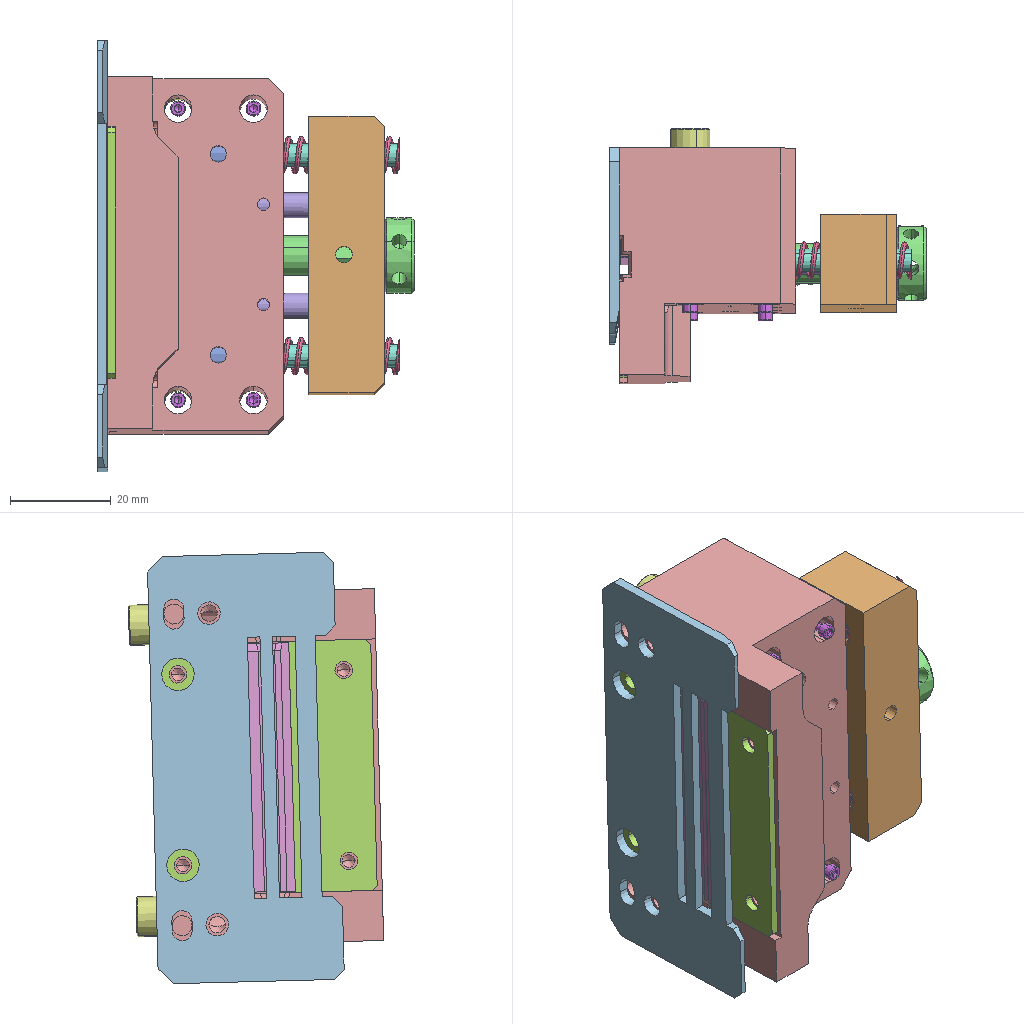Assembly | SolidWorks | 12 different items | 21 placed | box 63 x 51 x 86 mm
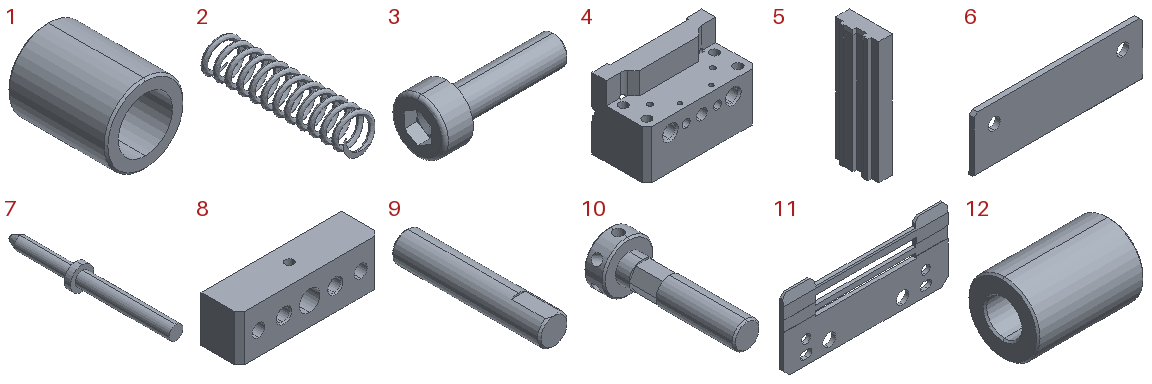Parts list (item | quantity | size | volume | features):
1 | x2 | 8 x 10 x 8 mm | 264.083 mm3 | features Chamfer 1, Extrusion 1
2 | x2 | 7.5 x 30 x 7.5 mm | 192.185 mm3 | features Helix 1, ICE 1, RefAxis 1, Sweep 1
3 | x4 | 7.6 x 3 x 3 mm | 21.652 mm3 | features Fillet 2, RevCut 2, Boss 1, Chamfer 1, Cut 1, Extrusion 1, LPattern 1
4 | x1 | 70 x 35 x 45 mm | 68698 mm3 | features ICE 23, Chamfer 5, HoleWzd 5, 3DProfileFeature 3, Cut 2, Extrusion 1, Fillet 1, LPattern 1, MirrorPattern 1
5 | x1 | 7 x 17.4 x 49.4 mm | 5230 mm3 | features ICE 3, Chamfer 2, RefAxis 2, Extrusion 1, MirrorPattern 1, RevCut 1
6 | x2 | 50 x 1.5 x 16.3 mm | 1186 mm3 | features Chamfer 2, Extrusion 1, ICE 1
7 | x2 | 7.5 x 53 x 7.5 mm | 808.158 mm3 | features ICE 3, Revolution 2, Extrusion 1, RefAxis 1, RevCut 1
8 | x1 | 55 x 15 x 18 mm | 12154 mm3 | features ICE 9, Chamfer 3, 3DProfileFeature 2, HoleWzd 2, Extrusion 1
9 | x2 | 5 x 25 x 5 mm | 486.718 mm3 | features Chamfer 1, Extrusion 1, ICE 1
10 | x1 | 15 x 41 x 15 mm | 2454 mm3 | features ICE 3, CirPattern 2, Chamfer 1, Extrusion 1
11 | x1 | 85 x 2 x 37 mm | 4721 mm3 | features ICE 7, Chamfer 5, Cut 2, Extrusion 1
12 | x2 | 12 x 8 x 8 mm | 450.881 mm3 | features RefAxis 3, 3DProfileFeature 1, Chamfer 1, Revolution 1
Mates (type | each side: item.copy, entity, surface, feature):
Coincident | 5.1 face plane Cut-Extrude3 | 6.1 face plane Boss-Extrude1
Coincident | 5.1 face plane Cut-Extrude3 | 6.2 face plane Boss-Extrude1
Coincident | 5.1 axis | 7.1 axis
Concentric | 5.1 face sphere Cut-Revolve1 | 7.2 face sphere Revolve1
Coincident | 7.1 face plane Boss-Extrude2 | 7.2 face plane Boss-Extrude2
Coincident | 7.1 face plane Boss-Extrude2 | 2.1 face plane Cut-Extrude1
Coincident | 7.1 axis | 2.1 axis
Coincident | 7.2 face plane Boss-Extrude2 | 2.2 face plane Cut-Extrude1
Coincident | 7.2 axis | 2.2 axis
Concentric | 8.1 face cylinder Ø8.2 (8.2) Diameter Hole1 | 10.1 face cylinder Boss-Extrude1
Coincident | 8.1 face plane Boss-Extrude1 | 10.1 face plane Boss-Extrude2
Coincident | 9.1 face plane Boss-Extrude1 | 9.2 face plane Boss-Extrude1
Coincident | 4.1 face plane Boss-Extrude11 | 12.1 face plane Revolve1
Coincident | 4.1 face plane Boss-Extrude11 | 12.2 face plane Revolve1
Concentric | 7.1 face cylinder Boss-Extrude3 | 4.1 face cylinder Cut-Extrude1
Concentric | 7.2 face cylinder Boss-Extrude3 | 4.1 face cylinder Cut-Extrude1
Concentric | 4.1 face cylinder Cut-Extrude1 | 8.1 face cylinder Cut-Extrude1 | 2 times
Concentric | 4.1 face cylinder Cut-Extrude4 | 9.1 face cylinder Boss-Extrude1
Concentric | 4.1 face cylinder Cut-Extrude4 | 9.2 face cylinder Boss-Extrude1
DistanceDim | 8.1 face plane Cut-Extrude7 | 4.1 face plane Boss-Extrude4
Coincident | 4.1 face plane Cut-Extrude4 | 9.1 face plane Boss-Extrude1
Coincident | 4.1 face plane Boss-Extrude8 | 11.1 face plane Boss-Extrude1
Concentric | 4.1 face cylinder Cut-Extrude13 | 3.1 face cylinder BaseBody
Coincident | 4.1 face plane Boss-Extrude3 | 3.1 face plane BaseHead
Concentric | 4.1 face cylinder Cut-Extrude13 | 3.2 face cylinder BaseBody
Coincident | 4.1 face plane Boss-Extrude3 | 3.2 face plane BaseHead
Concentric | 4.1 face cylinder LPattern1 | 3.3 face cylinder BaseBody
Coincident | 4.1 face plane Boss-Extrude3 | 3.3 face plane BaseHead
Concentric | 4.1 face cylinder LPattern1 | 3.4 face cylinder BaseBody
Coincident | 4.1 face plane Boss-Extrude3 | 3.4 face plane BaseHead
Concentric | 4.1 face cylinder M3 Tapped Hole2 | 6.1 face cylinder Cut-Extrude2 | 2 times
Coincident | 4.1 face plane Cut-Extrude17 | 1.1 face plane Boss-Extrude1
Concentric | 4.1 face cylinder Cut-Extrude17 | 1.1 face cylinder Boss-Extrude1
Coincident | 4.1 face plane Cut-Extrude17 | 1.2 face plane Boss-Extrude1
Concentric | 4.1 face cylinder Cut-Extrude17 | 1.2 face cylinder Boss-Extrude1
Concentric | 4.1 face cylinder M4 Tapped Hole2 | 11.1 face cylinder Cut-Extrude3 | 2 times
Concentric | 7.1 face cylinder Boss-Extrude3 | 12.2 face cylinder Revolve1
Concentric | 7.2 face cylinder Boss-Extrude3 | 12.1 face cylinder Revolve1
Coincident | 6.2 face plane Boss-Extrude1 | 5.1 face plane Cut-Extrude3
Concentric | 4.1 face cylinder M3 Tapped Hole2 | 6.2 face cylinder Cut-Extrude2 | 2 times
Coincident | 4.1 face plane Cut-Extrude10 | 6.2 face plane Boss-Extrude1